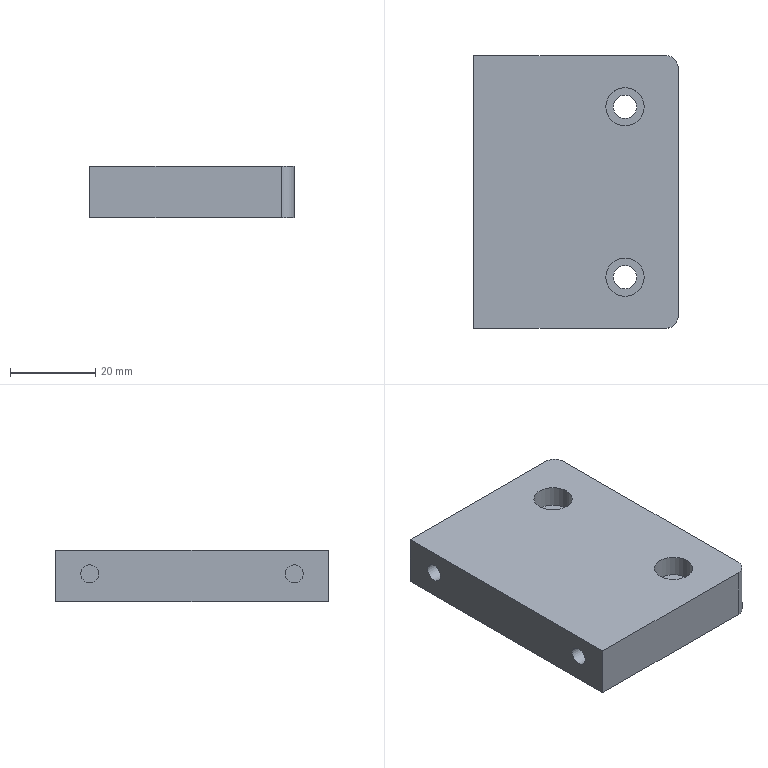Part | STEP file | ROTATION MC_NEW VER-0610_550 | 1 solid | 19 faces | box 48 x 64 x 12 mm | volume 35212 mm3 | plane 10 | cylinder 9 | commonest cylinder face diameters 5.5 x3 4.2 x2 6 x2 9 x2
STEP:
#1=CARTESIAN_POINT('',(378.531,390.468,-136.091));
#2=VERTEX_POINT('',#1);
#3=CARTESIAN_POINT('',(378.531,454.468,-136.091));
#4=VERTEX_POINT('',#3);
#5=CARTESIAN_POINT('',(378.531,390.468,-136.091));
#6=DIRECTION('',(0.,1.,0.));
#7=VECTOR('',#6,64.);
#8=LINE('',#5,#7);
#9=EDGE_CURVE('',#2,#4,#8,.T.);
#10=ORIENTED_EDGE('',*,*,#9,.F.);
#11=CARTESIAN_POINT('',(378.531,390.468,-124.091));
#12=VERTEX_POINT('',#11);
#13=CARTESIAN_POINT('',(378.531,390.468,-124.091));
#14=DIRECTION('',(0.,0.,-1.));
#15=VECTOR('',#14,12.);
#16=LINE('',#13,#15);
#17=EDGE_CURVE('',#12,#2,#16,.T.);
#18=ORIENTED_EDGE('',*,*,#17,.F.);
#19=CARTESIAN_POINT('',(378.531,454.468,-124.091));
#20=VERTEX_POINT('',#19);
#21=CARTESIAN_POINT('',(378.531,454.468,-124.091));
#22=DIRECTION('',(0.,-1.,0.));
#23=VECTOR('',#22,64.);
#24=LINE('',#21,#23);
#25=EDGE_CURVE('',#20,#12,#24,.T.);
#26=ORIENTED_EDGE('',*,*,#25,.F.);
#27=CARTESIAN_POINT('',(378.531,454.468,-136.091));
#28=DIRECTION('',(0.,0.,1.));
#29=VECTOR('',#28,12.);
#30=LINE('',#27,#29);
#31=EDGE_CURVE('',#4,#20,#30,.T.);
#32=ORIENTED_EDGE('',*,*,#31,.F.);
#33=EDGE_LOOP('',(#10,#18,#26,#32));
#34=FACE_OUTER_BOUND('',#33,.T.);
#35=CARTESIAN_POINT('',(378.531,448.568,-129.591));
#36=VERTEX_POINT('',#35);
#37=CARTESIAN_POINT('',(378.531,444.368,-129.591));
#38=VERTEX_POINT('',#37);
#39=CARTESIAN_POINT('',(378.531,446.468,-129.591));
#40=DIRECTION('',(1.,0.,0.));
#41=DIRECTION('',(0.,1.,0.));
#42=AXIS2_PLACEMENT_3D('',#39,#40,#41);
#43=CIRCLE('',#42,2.1);
#44=EDGE_CURVE('',#36,#38,#43,.T.);
#45=ORIENTED_EDGE('',*,*,#44,.T.);
#46=CARTESIAN_POINT('',(378.531,446.468,-129.591));
#47=DIRECTION('',(1.,0.,0.));
#48=DIRECTION('',(0.,1.,0.));
#49=AXIS2_PLACEMENT_3D('',#46,#47,#48);
#50=CIRCLE('',#49,2.1);
#51=EDGE_CURVE('',#38,#36,#50,.T.);
#52=ORIENTED_EDGE('',*,*,#51,.T.);
#53=EDGE_LOOP('',(#45,#52));
#54=FACE_BOUND('',#53,.T.);
#55=CARTESIAN_POINT('',(378.531,400.568,-129.591));
#56=VERTEX_POINT('',#55);
#57=CARTESIAN_POINT('',(378.531,396.368,-129.591));
#58=VERTEX_POINT('',#57);
#59=CARTESIAN_POINT('',(378.531,398.468,-129.591));
#60=DIRECTION('',(1.,0.,0.));
#61=DIRECTION('',(0.,1.,0.));
#62=AXIS2_PLACEMENT_3D('',#59,#60,#61);
#63=CIRCLE('',#62,2.1);
#64=EDGE_CURVE('',#56,#58,#63,.T.);
#65=ORIENTED_EDGE('',*,*,#64,.T.);
#66=CARTESIAN_POINT('',(378.531,398.468,-129.591));
#67=DIRECTION('',(1.,0.,0.));
#68=DIRECTION('',(0.,1.,0.));
#69=AXIS2_PLACEMENT_3D('',#66,#67,#68);
#70=CIRCLE('',#69,2.1);
#71=EDGE_CURVE('',#58,#56,#70,.T.);
#72=ORIENTED_EDGE('',*,*,#71,.T.);
#73=EDGE_LOOP('',(#65,#72));
#74=FACE_BOUND('',#73,.T.);
#75=CARTESIAN_POINT('',(378.531,397.468,-97.591));
#76=DIRECTION('',(1.,0.,0.));
#77=DIRECTION('',(0.,0.,-1.));
#78=AXIS2_PLACEMENT_3D('',#75,#76,#77);
#79=PLANE('',#78);
#80=ADVANCED_FACE('',(#34,#54,#74),#79,.F.);
#81=CARTESIAN_POINT('',(423.531,454.468,-136.091));
#82=VERTEX_POINT('',#81);
#83=CARTESIAN_POINT('',(426.531,451.468,-136.091));
#84=VERTEX_POINT('',#83);
#85=CARTESIAN_POINT('',(423.531,451.468,-136.091));
#86=DIRECTION('',(0.,0.,-1.));
#87=DIRECTION('',(0.7071,0.7071,0.));
#88=AXIS2_PLACEMENT_3D('',#85,#86,#87);
#89=CIRCLE('',#88,3.);
#90=EDGE_CURVE('',#82,#84,#89,.T.);
#91=ORIENTED_EDGE('',*,*,#90,.T.);
#92=CARTESIAN_POINT('',(426.531,393.468,-136.091));
#93=VERTEX_POINT('',#92);
#94=CARTESIAN_POINT('',(426.531,393.468,-136.091));
#95=DIRECTION('',(0.,1.,0.));
#96=VECTOR('',#95,58.);
#97=LINE('',#94,#96);
#98=EDGE_CURVE('',#93,#84,#97,.T.);
#99=ORIENTED_EDGE('',*,*,#98,.F.);
#100=CARTESIAN_POINT('',(423.531,390.468,-136.091));
#101=VERTEX_POINT('',#100);
#102=CARTESIAN_POINT('',(423.531,393.468,-136.091));
#103=DIRECTION('',(0.,0.,-1.));
#104=DIRECTION('',(1.,0.,0.));
#105=AXIS2_PLACEMENT_3D('',#102,#103,#104);
#106=CIRCLE('',#105,3.);
#107=EDGE_CURVE('',#93,#101,#106,.T.);
#108=ORIENTED_EDGE('',*,*,#107,.T.);
#109=CARTESIAN_POINT('',(423.531,390.468,-136.091));
#110=DIRECTION('',(-1.,0.,0.));
#111=VECTOR('',#110,45.);
#112=LINE('',#109,#111);
#113=EDGE_CURVE('',#101,#2,#112,.T.);
#114=ORIENTED_EDGE('',*,*,#113,.T.);
#115=ORIENTED_EDGE('',*,*,#9,.T.);
#116=CARTESIAN_POINT('',(378.531,454.468,-136.091));
#117=DIRECTION('',(1.,0.,0.));
#118=VECTOR('',#117,45.);
#119=LINE('',#116,#118);
#120=EDGE_CURVE('',#4,#82,#119,.T.);
#121=ORIENTED_EDGE('',*,*,#120,.T.);
#122=EDGE_LOOP('',(#91,#99,#108,#114,#115,#121));
#123=FACE_OUTER_BOUND('',#122,.T.);
#124=CARTESIAN_POINT('',(416.781,402.468,-136.091));
#125=VERTEX_POINT('',#124);
#126=CARTESIAN_POINT('',(414.031,402.468,-136.091));
#127=DIRECTION('',(0.,0.,1.));
#128=DIRECTION('',(-1.,0.,0.));
#129=AXIS2_PLACEMENT_3D('',#126,#127,#128);
#130=CIRCLE('',#129,2.75);
#131=EDGE_CURVE('',#125,#125,#130,.T.);
#132=ORIENTED_EDGE('',*,*,#131,.T.);
#133=EDGE_LOOP('',(#132));
#134=FACE_BOUND('',#133,.T.);
#135=CARTESIAN_POINT('',(416.781,442.468,-136.091));
#136=VERTEX_POINT('',#135);
#137=CARTESIAN_POINT('',(411.281,442.468,-136.091));
#138=VERTEX_POINT('',#137);
#139=CARTESIAN_POINT('',(414.031,442.468,-136.091));
#140=DIRECTION('',(0.,0.,1.));
#141=DIRECTION('',(-1.,0.,0.));
#142=AXIS2_PLACEMENT_3D('',#139,#140,#141);
#143=CIRCLE('',#142,2.75);
#144=EDGE_CURVE('',#136,#138,#143,.T.);
#145=ORIENTED_EDGE('',*,*,#144,.T.);
#146=CARTESIAN_POINT('',(414.031,442.468,-136.091));
#147=DIRECTION('',(0.,0.,1.));
#148=DIRECTION('',(-1.,0.,0.));
#149=AXIS2_PLACEMENT_3D('',#146,#147,#148);
#150=CIRCLE('',#149,2.75);
#151=EDGE_CURVE('',#138,#136,#150,.T.);
#152=ORIENTED_EDGE('',*,*,#151,.T.);
#153=EDGE_LOOP('',(#145,#152));
#154=FACE_BOUND('',#153,.T.);
#155=CARTESIAN_POINT('',(391.531,422.468,-136.091));
#156=DIRECTION('',(0.,0.,-1.));
#157=DIRECTION('',(-1.,0.,0.));
#158=AXIS2_PLACEMENT_3D('',#155,#156,#157);
#159=PLANE('',#158);
#160=ADVANCED_FACE('',(#123,#134,#154),#159,.T.);
#161=CARTESIAN_POINT('',(426.531,451.468,-124.091));
#162=VERTEX_POINT('',#161);
#163=CARTESIAN_POINT('',(423.531,454.468,-124.091));
#164=VERTEX_POINT('',#163);
#165=CARTESIAN_POINT('',(423.531,451.468,-124.091));
#166=DIRECTION('',(0.,0.,1.));
#167=DIRECTION('',(1.,0.,0.));
#168=AXIS2_PLACEMENT_3D('',#165,#166,#167);
#169=CIRCLE('',#168,3.);
#170=EDGE_CURVE('',#162,#164,#169,.T.);
#171=ORIENTED_EDGE('',*,*,#170,.F.);
#172=CARTESIAN_POINT('',(426.531,451.468,-124.091));
#173=DIRECTION('',(0.,0.,-1.));
#174=VECTOR('',#173,12.);
#175=LINE('',#172,#174);
#176=EDGE_CURVE('',#162,#84,#175,.T.);
#177=ORIENTED_EDGE('',*,*,#176,.T.);
#178=ORIENTED_EDGE('',*,*,#90,.F.);
#179=CARTESIAN_POINT('',(423.531,454.468,-136.091));
#180=DIRECTION('',(0.,0.,1.));
#181=VECTOR('',#180,12.);
#182=LINE('',#179,#181);
#183=EDGE_CURVE('',#82,#164,#182,.T.);
#184=ORIENTED_EDGE('',*,*,#183,.T.);
#185=EDGE_LOOP('',(#171,#177,#178,#184));
#186=FACE_OUTER_BOUND('',#185,.T.);
#187=CARTESIAN_POINT('',(423.531,451.468,-111.841));
#188=DIRECTION('',(0.,0.,-1.));
#189=DIRECTION('',(0.7071,0.7071,0.));
#190=AXIS2_PLACEMENT_3D('',#187,#188,#189);
#191=CYLINDRICAL_SURFACE('',#190,3.);
#192=ADVANCED_FACE('',(#186),#191,.T.);
#193=CARTESIAN_POINT('',(411.281,442.468,-129.091));
#194=VERTEX_POINT('',#193);
#195=CARTESIAN_POINT('',(416.781,442.468,-129.091));
#196=VERTEX_POINT('',#195);
#197=CARTESIAN_POINT('',(414.031,442.468,-129.091));
#198=DIRECTION('',(0.,0.,-1.));
#199=DIRECTION('',(-1.,0.,0.));
#200=AXIS2_PLACEMENT_3D('',#197,#198,#199);
#201=CIRCLE('',#200,2.75);
#202=EDGE_CURVE('',#194,#196,#201,.T.);
#203=ORIENTED_EDGE('',*,*,#202,.F.);
#204=CARTESIAN_POINT('',(411.281,442.468,-136.091));
#205=DIRECTION('',(0.,0.,1.));
#206=VECTOR('',#205,7.);
#207=LINE('',#204,#206);
#208=EDGE_CURVE('',#138,#194,#207,.T.);
#209=ORIENTED_EDGE('',*,*,#208,.F.);
#210=ORIENTED_EDGE('',*,*,#144,.F.);
#211=CARTESIAN_POINT('',(416.781,442.468,-136.091));
#212=DIRECTION('',(0.,0.,1.));
#213=VECTOR('',#212,7.);
#214=LINE('',#211,#213);
#215=EDGE_CURVE('',#136,#196,#214,.T.);
#216=ORIENTED_EDGE('',*,*,#215,.T.);
#217=EDGE_LOOP('',(#203,#209,#210,#216));
#218=FACE_OUTER_BOUND('',#217,.T.);
#219=CARTESIAN_POINT('',(414.031,442.468,-120.091));
#220=DIRECTION('',(0.,0.,-1.));
#221=DIRECTION('',(-1.,0.,0.));
#222=AXIS2_PLACEMENT_3D('',#219,#220,#221);
#223=CYLINDRICAL_SURFACE('',#222,2.75);
#224=ADVANCED_FACE('',(#218),#223,.F.);
#225=ORIENTED_EDGE('',*,*,#170,.T.);
#226=CARTESIAN_POINT('',(423.531,454.468,-124.091));
#227=DIRECTION('',(-1.,0.,0.));
#228=VECTOR('',#227,45.);
#229=LINE('',#226,#228);
#230=EDGE_CURVE('',#164,#20,#229,.T.);
#231=ORIENTED_EDGE('',*,*,#230,.T.);
#232=ORIENTED_EDGE('',*,*,#25,.T.);
#233=CARTESIAN_POINT('',(423.531,390.468,-124.091));
#234=VERTEX_POINT('',#233);
#235=CARTESIAN_POINT('',(423.531,390.468,-124.091));
#236=DIRECTION('',(-1.,0.,0.));
#237=VECTOR('',#236,45.);
#238=LINE('',#235,#237);
#239=EDGE_CURVE('',#234,#12,#238,.T.);
#240=ORIENTED_EDGE('',*,*,#239,.F.);
#241=CARTESIAN_POINT('',(426.531,393.468,-124.091));
#242=VERTEX_POINT('',#241);
#243=CARTESIAN_POINT('',(423.531,393.468,-124.091));
#244=DIRECTION('',(0.,0.,1.));
#245=DIRECTION('',(0.,-1.,0.));
#246=AXIS2_PLACEMENT_3D('',#243,#244,#245);
#247=CIRCLE('',#246,3.);
#248=EDGE_CURVE('',#234,#242,#247,.T.);
#249=ORIENTED_EDGE('',*,*,#248,.T.);
#250=CARTESIAN_POINT('',(426.531,451.468,-124.091));
#251=DIRECTION('',(0.,-1.,0.));
#252=VECTOR('',#251,58.);
#253=LINE('',#250,#252);
#254=EDGE_CURVE('',#162,#242,#253,.T.);
#255=ORIENTED_EDGE('',*,*,#254,.F.);
#256=EDGE_LOOP('',(#225,#231,#232,#240,#249,#255));
#257=FACE_OUTER_BOUND('',#256,.T.);
#258=CARTESIAN_POINT('',(409.531,402.468,-124.091));
#259=VERTEX_POINT('',#258);
#260=CARTESIAN_POINT('',(418.531,402.468,-124.091));
#261=VERTEX_POINT('',#260);
#262=CARTESIAN_POINT('',(414.031,402.468,-124.091));
#263=DIRECTION('',(0.,0.,-1.));
#264=DIRECTION('',(-1.,0.,0.));
#265=AXIS2_PLACEMENT_3D('',#262,#263,#264);
#266=CIRCLE('',#265,4.5);
#267=EDGE_CURVE('',#259,#261,#266,.T.);
#268=ORIENTED_EDGE('',*,*,#267,.T.);
#269=CARTESIAN_POINT('',(414.031,402.468,-124.091));
#270=DIRECTION('',(0.,0.,-1.));
#271=DIRECTION('',(-1.,0.,0.));
#272=AXIS2_PLACEMENT_3D('',#269,#270,#271);
#273=CIRCLE('',#272,4.5);
#274=EDGE_CURVE('',#261,#259,#273,.T.);
#275=ORIENTED_EDGE('',*,*,#274,.T.);
#276=EDGE_LOOP('',(#268,#275));
#277=FACE_BOUND('',#276,.T.);
#278=CARTESIAN_POINT('',(409.531,442.468,-124.091));
#279=VERTEX_POINT('',#278);
#280=CARTESIAN_POINT('',(418.531,442.468,-124.091));
#281=VERTEX_POINT('',#280);
#282=CARTESIAN_POINT('',(414.031,442.468,-124.091));
#283=DIRECTION('',(0.,0.,-1.));
#284=DIRECTION('',(1.,0.,0.));
#285=AXIS2_PLACEMENT_3D('',#282,#283,#284);
#286=CIRCLE('',#285,4.5);
#287=EDGE_CURVE('',#279,#281,#286,.T.);
#288=ORIENTED_EDGE('',*,*,#287,.T.);
#289=CARTESIAN_POINT('',(414.031,442.468,-124.091));
#290=DIRECTION('',(0.,0.,-1.));
#291=DIRECTION('',(1.,0.,0.));
#292=AXIS2_PLACEMENT_3D('',#289,#290,#291);
#293=CIRCLE('',#292,4.5);
#294=EDGE_CURVE('',#281,#279,#293,.T.);
#295=ORIENTED_EDGE('',*,*,#294,.T.);
#296=EDGE_LOOP('',(#288,#295));
#297=FACE_BOUND('',#296,.T.);
#298=CARTESIAN_POINT('',(391.531,422.468,-124.091));
#299=DIRECTION('',(0.,0.,1.));
#300=DIRECTION('',(1.,0.,0.));
#301=AXIS2_PLACEMENT_3D('',#298,#299,#300);
#302=PLANE('',#301);
#303=ADVANCED_FACE('',(#257,#277,#297),#302,.T.);
#304=ORIENTED_EDGE('',*,*,#176,.F.);
#305=ORIENTED_EDGE('',*,*,#254,.T.);
#306=CARTESIAN_POINT('',(426.531,393.468,-136.091));
#307=DIRECTION('',(0.,0.,1.));
#308=VECTOR('',#307,12.);
#309=LINE('',#306,#308);
#310=EDGE_CURVE('',#93,#242,#309,.T.);
#311=ORIENTED_EDGE('',*,*,#310,.F.);
#312=ORIENTED_EDGE('',*,*,#98,.T.);
#313=EDGE_LOOP('',(#304,#305,#311,#312));
#314=FACE_OUTER_BOUND('',#313,.T.);
#315=CARTESIAN_POINT('',(426.531,397.468,-97.591));
#316=DIRECTION('',(1.,0.,0.));
#317=DIRECTION('',(0.,0.,-1.));
#318=AXIS2_PLACEMENT_3D('',#315,#316,#317);
#319=PLANE('',#318);
#320=ADVANCED_FACE('',(#314),#319,.T.);
#321=ORIENTED_EDGE('',*,*,#107,.F.);
#322=ORIENTED_EDGE('',*,*,#310,.T.);
#323=ORIENTED_EDGE('',*,*,#248,.F.);
#324=CARTESIAN_POINT('',(423.531,390.468,-124.091));
#325=DIRECTION('',(0.,0.,-1.));
#326=VECTOR('',#325,12.);
#327=LINE('',#324,#326);
#328=EDGE_CURVE('',#234,#101,#327,.T.);
#329=ORIENTED_EDGE('',*,*,#328,.T.);
#330=EDGE_LOOP('',(#321,#322,#323,#329));
#331=FACE_OUTER_BOUND('',#330,.T.);
#332=CARTESIAN_POINT('',(423.531,393.468,-111.841));
#333=DIRECTION('',(0.,0.,1.));
#334=DIRECTION('',(0.7071,-0.7071,0.));
#335=AXIS2_PLACEMENT_3D('',#332,#333,#334);
#336=CYLINDRICAL_SURFACE('',#335,3.);
#337=ADVANCED_FACE('',(#331),#336,.T.);
#338=CARTESIAN_POINT('',(401.531,448.568,-129.591));
#339=VERTEX_POINT('',#338);
#340=CARTESIAN_POINT('',(401.531,444.368,-129.591));
#341=VERTEX_POINT('',#340);
#342=CARTESIAN_POINT('',(401.531,446.468,-129.591));
#343=DIRECTION('',(-1.,0.,0.));
#344=DIRECTION('',(0.,-1.,0.));
#345=AXIS2_PLACEMENT_3D('',#342,#343,#344);
#346=CIRCLE('',#345,2.1);
#347=EDGE_CURVE('',#339,#341,#346,.T.);
#348=ORIENTED_EDGE('',*,*,#347,.T.);
#349=CARTESIAN_POINT('',(401.531,446.468,-129.591));
#350=DIRECTION('',(-1.,0.,0.));
#351=DIRECTION('',(0.,-1.,0.));
#352=AXIS2_PLACEMENT_3D('',#349,#350,#351);
#353=CIRCLE('',#352,2.1);
#354=EDGE_CURVE('',#341,#339,#353,.T.);
#355=ORIENTED_EDGE('',*,*,#354,.T.);
#356=EDGE_LOOP('',(#348,#355));
#357=FACE_OUTER_BOUND('',#356,.T.);
#358=CARTESIAN_POINT('',(401.531,422.028,-97.591));
#359=DIRECTION('',(1.,0.,0.));
#360=DIRECTION('',(0.,0.,-1.));
#361=AXIS2_PLACEMENT_3D('',#358,#359,#360);
#362=PLANE('',#361);
#363=ADVANCED_FACE('',(#357),#362,.F.);
#364=ORIENTED_EDGE('',*,*,#328,.F.);
#365=ORIENTED_EDGE('',*,*,#239,.T.);
#366=ORIENTED_EDGE('',*,*,#17,.T.);
#367=ORIENTED_EDGE('',*,*,#113,.F.);
#368=EDGE_LOOP('',(#364,#365,#366,#367));
#369=FACE_OUTER_BOUND('',#368,.T.);
#370=CARTESIAN_POINT('',(391.531,390.468,-126.091));
#371=DIRECTION('',(0.,-1.,0.));
#372=DIRECTION('',(0.,0.,-1.));
#373=AXIS2_PLACEMENT_3D('',#370,#371,#372);
#374=PLANE('',#373);
#375=ADVANCED_FACE('',(#369),#374,.T.);
#376=ORIENTED_EDGE('',*,*,#183,.F.);
#377=ORIENTED_EDGE('',*,*,#120,.F.);
#378=ORIENTED_EDGE('',*,*,#31,.T.);
#379=ORIENTED_EDGE('',*,*,#230,.F.);
#380=EDGE_LOOP('',(#376,#377,#378,#379));
#381=FACE_OUTER_BOUND('',#380,.T.);
#382=CARTESIAN_POINT('',(391.531,454.468,-126.091));
#383=DIRECTION('',(0.,1.,0.));
#384=DIRECTION('',(0.,0.,1.));
#385=AXIS2_PLACEMENT_3D('',#382,#383,#384);
#386=PLANE('',#385);
#387=ADVANCED_FACE('',(#381),#386,.T.);
#388=ORIENTED_EDGE('',*,*,#267,.F.);
#389=ORIENTED_EDGE('',*,*,#274,.F.);
#390=CARTESIAN_POINT('',(418.531,402.468,-129.091));
#391=VERTEX_POINT('',#390);
#392=CARTESIAN_POINT('',(418.531,402.468,-120.091));
#393=DIRECTION('',(0.,0.,-1.));
#394=VECTOR('',#393,4.5);
#395=LINE('',#392,#394);
#396=EDGE_CURVE('',#261,#391,#395,.T.);
#397=ORIENTED_EDGE('',*,*,#396,.T.);
#398=CARTESIAN_POINT('',(409.531,402.468,-129.091));
#399=VERTEX_POINT('',#398);
#400=CARTESIAN_POINT('',(414.031,402.468,-129.091));
#401=DIRECTION('',(0.,0.,1.));
#402=DIRECTION('',(1.,0.,0.));
#403=AXIS2_PLACEMENT_3D('',#400,#401,#402);
#404=CIRCLE('',#403,4.5);
#405=EDGE_CURVE('',#399,#391,#404,.T.);
#406=ORIENTED_EDGE('',*,*,#405,.F.);
#407=CARTESIAN_POINT('',(414.031,402.468,-129.091));
#408=DIRECTION('',(0.,0.,1.));
#409=DIRECTION('',(1.,0.,0.));
#410=AXIS2_PLACEMENT_3D('',#407,#408,#409);
#411=CIRCLE('',#410,4.5);
#412=EDGE_CURVE('',#391,#399,#411,.T.);
#413=ORIENTED_EDGE('',*,*,#412,.F.);
#414=ORIENTED_EDGE('',*,*,#396,.F.);
#415=EDGE_LOOP('',(#388,#389,#397,#406,#413,#414));
#416=FACE_OUTER_BOUND('',#415,.T.);
#417=CARTESIAN_POINT('',(414.031,402.468,-120.091));
#418=DIRECTION('',(0.,0.,-1.));
#419=DIRECTION('',(-1.,0.,0.));
#420=AXIS2_PLACEMENT_3D('',#417,#418,#419);
#421=CYLINDRICAL_SURFACE('',#420,4.5);
#422=ADVANCED_FACE('',(#416),#421,.F.);
#423=CARTESIAN_POINT('',(401.531,400.568,-129.591));
#424=VERTEX_POINT('',#423);
#425=CARTESIAN_POINT('',(401.531,396.368,-129.591));
#426=VERTEX_POINT('',#425);
#427=CARTESIAN_POINT('',(401.531,398.468,-129.591));
#428=DIRECTION('',(-1.,0.,0.));
#429=DIRECTION('',(0.,-1.,0.));
#430=AXIS2_PLACEMENT_3D('',#427,#428,#429);
#431=CIRCLE('',#430,2.1);
#432=EDGE_CURVE('',#424,#426,#431,.T.);
#433=ORIENTED_EDGE('',*,*,#432,.T.);
#434=CARTESIAN_POINT('',(401.531,398.468,-129.591));
#435=DIRECTION('',(-1.,0.,0.));
#436=DIRECTION('',(0.,-1.,0.));
#437=AXIS2_PLACEMENT_3D('',#434,#435,#436);
#438=CIRCLE('',#437,2.1);
#439=EDGE_CURVE('',#426,#424,#438,.T.);
#440=ORIENTED_EDGE('',*,*,#439,.T.);
#441=EDGE_LOOP('',(#433,#440));
#442=FACE_OUTER_BOUND('',#441,.T.);
#443=CARTESIAN_POINT('',(401.531,374.858,-97.591));
#444=DIRECTION('',(1.,0.,0.));
#445=DIRECTION('',(0.,0.,-1.));
#446=AXIS2_PLACEMENT_3D('',#443,#444,#445);
#447=PLANE('',#446);
#448=ADVANCED_FACE('',(#442),#447,.F.);
#449=ORIENTED_EDGE('',*,*,#405,.T.);
#450=ORIENTED_EDGE('',*,*,#412,.T.);
#451=EDGE_LOOP('',(#449,#450));
#452=FACE_OUTER_BOUND('',#451,.T.);
#453=CARTESIAN_POINT('',(416.781,402.468,-129.091));
#454=VERTEX_POINT('',#453);
#455=CARTESIAN_POINT('',(414.031,402.468,-129.091));
#456=DIRECTION('',(0.,0.,-1.));
#457=DIRECTION('',(1.,0.,0.));
#458=AXIS2_PLACEMENT_3D('',#455,#456,#457);
#459=CIRCLE('',#458,2.75);
#460=EDGE_CURVE('',#454,#454,#459,.T.);
#461=ORIENTED_EDGE('',*,*,#460,.T.);
#462=EDGE_LOOP('',(#461));
#463=FACE_BOUND('',#462,.T.);
#464=CARTESIAN_POINT('',(411.781,402.468,-129.091));
#465=DIRECTION('',(0.,0.,1.));
#466=DIRECTION('',(1.,0.,0.));
#467=AXIS2_PLACEMENT_3D('',#464,#465,#466);
#468=PLANE('',#467);
#469=ADVANCED_FACE('',(#452,#463),#468,.T.);
#470=ORIENTED_EDGE('',*,*,#460,.F.);
#471=CARTESIAN_POINT('',(416.781,402.468,-120.091));
#472=DIRECTION('',(0.,0.,-1.));
#473=VECTOR('',#472,2.75);
#474=LINE('',#471,#473);
#475=EDGE_CURVE('',#454,#125,#474,.T.);
#476=ORIENTED_EDGE('',*,*,#475,.T.);
#477=ORIENTED_EDGE('',*,*,#131,.F.);
#478=ORIENTED_EDGE('',*,*,#475,.F.);
#479=EDGE_LOOP('',(#470,#476,#477,#478));
#480=FACE_OUTER_BOUND('',#479,.T.);
#481=CARTESIAN_POINT('',(414.031,402.468,-120.091));
#482=DIRECTION('',(0.,0.,-1.));
#483=DIRECTION('',(-1.,0.,0.));
#484=AXIS2_PLACEMENT_3D('',#481,#482,#483);
#485=CYLINDRICAL_SURFACE('',#484,2.75);
#486=ADVANCED_FACE('',(#480),#485,.F.);
#487=ORIENTED_EDGE('',*,*,#432,.F.);
#488=ORIENTED_EDGE('',*,*,#439,.F.);
#489=CARTESIAN_POINT('',(384.531,396.368,-129.591));
#490=DIRECTION('',(-1.,0.,0.));
#491=VECTOR('',#490,2.1);
#492=LINE('',#489,#491);
#493=EDGE_CURVE('',#426,#58,#492,.T.);
#494=ORIENTED_EDGE('',*,*,#493,.T.);
#495=ORIENTED_EDGE('',*,*,#64,.F.);
#496=ORIENTED_EDGE('',*,*,#71,.F.);
#497=ORIENTED_EDGE('',*,*,#493,.F.);
#498=EDGE_LOOP('',(#487,#488,#494,#495,#496,#497));
#499=FACE_OUTER_BOUND('',#498,.T.);
#500=CARTESIAN_POINT('',(384.531,398.468,-129.591));
#501=DIRECTION('',(-1.,0.,0.));
#502=DIRECTION('',(0.,1.,0.));
#503=AXIS2_PLACEMENT_3D('',#500,#501,#502);
#504=CYLINDRICAL_SURFACE('',#503,2.1);
#505=ADVANCED_FACE('',(#499),#504,.F.);
#506=ORIENTED_EDGE('',*,*,#287,.F.);
#507=ORIENTED_EDGE('',*,*,#294,.F.);
#508=CARTESIAN_POINT('',(418.531,442.468,-129.091));
#509=VERTEX_POINT('',#508);
#510=CARTESIAN_POINT('',(418.531,442.468,-120.091));
#511=DIRECTION('',(0.,0.,-1.));
#512=VECTOR('',#511,4.5);
#513=LINE('',#510,#512);
#514=EDGE_CURVE('',#281,#509,#513,.T.);
#515=ORIENTED_EDGE('',*,*,#514,.T.);
#516=CARTESIAN_POINT('',(409.531,442.468,-129.091));
#517=VERTEX_POINT('',#516);
#518=CARTESIAN_POINT('',(414.031,442.468,-129.091));
#519=DIRECTION('',(0.,0.,1.));
#520=DIRECTION('',(-1.,0.,0.));
#521=AXIS2_PLACEMENT_3D('',#518,#519,#520);
#522=CIRCLE('',#521,4.5);
#523=EDGE_CURVE('',#517,#509,#522,.T.);
#524=ORIENTED_EDGE('',*,*,#523,.F.);
#525=CARTESIAN_POINT('',(414.031,442.468,-129.091));
#526=DIRECTION('',(0.,0.,1.));
#527=DIRECTION('',(-1.,0.,0.));
#528=AXIS2_PLACEMENT_3D('',#525,#526,#527);
#529=CIRCLE('',#528,4.5);
#530=EDGE_CURVE('',#509,#517,#529,.T.);
#531=ORIENTED_EDGE('',*,*,#530,.F.);
#532=ORIENTED_EDGE('',*,*,#514,.F.);
#533=EDGE_LOOP('',(#506,#507,#515,#524,#531,#532));
#534=FACE_OUTER_BOUND('',#533,.T.);
#535=CARTESIAN_POINT('',(414.031,442.468,-120.091));
#536=DIRECTION('',(0.,0.,-1.));
#537=DIRECTION('',(-1.,0.,0.));
#538=AXIS2_PLACEMENT_3D('',#535,#536,#537);
#539=CYLINDRICAL_SURFACE('',#538,4.5);
#540=ADVANCED_FACE('',(#534),#539,.F.);
#541=ORIENTED_EDGE('',*,*,#347,.F.);
#542=ORIENTED_EDGE('',*,*,#354,.F.);
#543=CARTESIAN_POINT('',(384.531,444.368,-129.591));
#544=DIRECTION('',(-1.,0.,0.));
#545=VECTOR('',#544,2.1);
#546=LINE('',#543,#545);
#547=EDGE_CURVE('',#341,#38,#546,.T.);
#548=ORIENTED_EDGE('',*,*,#547,.T.);
#549=ORIENTED_EDGE('',*,*,#44,.F.);
#550=ORIENTED_EDGE('',*,*,#51,.F.);
#551=ORIENTED_EDGE('',*,*,#547,.F.);
#552=EDGE_LOOP('',(#541,#542,#548,#549,#550,#551));
#553=FACE_OUTER_BOUND('',#552,.T.);
#554=CARTESIAN_POINT('',(384.531,446.468,-129.591));
#555=DIRECTION('',(-1.,0.,0.));
#556=DIRECTION('',(0.,1.,0.));
#557=AXIS2_PLACEMENT_3D('',#554,#555,#556);
#558=CYLINDRICAL_SURFACE('',#557,2.1);
#559=ADVANCED_FACE('',(#553),#558,.F.);
#560=ORIENTED_EDGE('',*,*,#523,.T.);
#561=ORIENTED_EDGE('',*,*,#530,.T.);
#562=EDGE_LOOP('',(#560,#561));
#563=FACE_OUTER_BOUND('',#562,.T.);
#564=ORIENTED_EDGE('',*,*,#202,.T.);
#565=CARTESIAN_POINT('',(414.031,442.468,-129.091));
#566=DIRECTION('',(0.,0.,-1.));
#567=DIRECTION('',(-1.,0.,0.));
#568=AXIS2_PLACEMENT_3D('',#565,#566,#567);
#569=CIRCLE('',#568,2.75);
#570=EDGE_CURVE('',#196,#194,#569,.T.);
#571=ORIENTED_EDGE('',*,*,#570,.T.);
#572=EDGE_LOOP('',(#564,#571));
#573=FACE_BOUND('',#572,.T.);
#574=CARTESIAN_POINT('',(411.781,442.468,-129.091));
#575=DIRECTION('',(0.,0.,1.));
#576=DIRECTION('',(1.,0.,0.));
#577=AXIS2_PLACEMENT_3D('',#574,#575,#576);
#578=PLANE('',#577);
#579=ADVANCED_FACE('',(#563,#573),#578,.T.);
#580=ORIENTED_EDGE('',*,*,#215,.F.);
#581=ORIENTED_EDGE('',*,*,#151,.F.);
#582=ORIENTED_EDGE('',*,*,#208,.T.);
#583=ORIENTED_EDGE('',*,*,#570,.F.);
#584=EDGE_LOOP('',(#580,#581,#582,#583));
#585=FACE_OUTER_BOUND('',#584,.T.);
#586=CARTESIAN_POINT('',(414.031,442.468,-120.091));
#587=DIRECTION('',(0.,0.,-1.));
#588=DIRECTION('',(-1.,0.,0.));
#589=AXIS2_PLACEMENT_3D('',#586,#587,#588);
#590=CYLINDRICAL_SURFACE('',#589,2.75);
#591=ADVANCED_FACE('',(#585),#590,.F.);
#592=CLOSED_SHELL('',(#80,#160,#192,#224,#303,#320,#337,#363,#375,#387,#422,#448,#469,#486,#505,#540,#559,#579,#591));
#593=MANIFOLD_SOLID_BREP('',#592);
#594=(LENGTH_UNIT()NAMED_UNIT(*)SI_UNIT(.MILLI.,.METRE.));
#595=UNCERTAINTY_MEASURE_WITH_UNIT(LENGTH_MEASURE(0.01),#594,'','');
#596=(NAMED_UNIT(*)PLANE_ANGLE_UNIT()SI_UNIT($,.RADIAN.));
#597=(NAMED_UNIT(*)SI_UNIT($,.STERADIAN.)SOLID_ANGLE_UNIT());
#598=(GEOMETRIC_REPRESENTATION_CONTEXT(3)GLOBAL_UNCERTAINTY_ASSIGNED_CONTEXT((#595))GLOBAL_UNIT_ASSIGNED_CONTEXT((#594,#596,#597))REPRESENTATION_CONTEXT('',''));
#599=ADVANCED_BREP_SHAPE_REPRESENTATION('',(#593),#598);